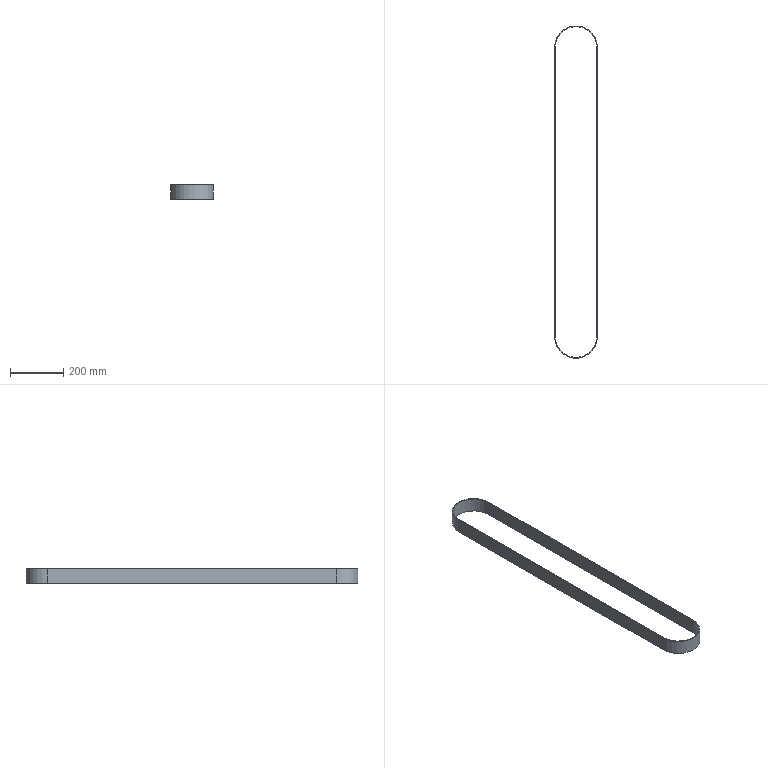Part | STEP file | timing belt 14M-2660L_default | 1 solid | 10 faces | box 161.176 x 1246 x 55 mm | volume 381989 mm3 | plane 6 | cylinder 4 | commonest cylinder face diameters 155.97 x2 161.176 x2
STEP:
#1=CARTESIAN_POINT('',(0.,0.,0.));
#2=DIRECTION('',(0.,0.,1.));
#3=DIRECTION('',(1.,0.,0.));
#4=AXIS2_PLACEMENT_3D('',#1,#2,#3);
#5=CARTESIAN_POINT('',(80.588,0.,-35.));
#6=VERTEX_POINT('',#5);
#7=CARTESIAN_POINT('',(-80.588,0.,-35.));
#8=VERTEX_POINT('',#7);
#9=CARTESIAN_POINT('',(0.,0.,-35.));
#10=DIRECTION('',(0.,0.,-1.));
#11=DIRECTION('',(-1.,0.,0.));
#12=AXIS2_PLACEMENT_3D('',#9,#10,#11);
#13=CIRCLE('',#12,80.588);
#14=CARTESIAN_POINT('',(0.,0.,20.));
#15=DIRECTION('',(0.,0.,-1.));
#16=DIRECTION('',(-1.,0.,0.));
#17=AXIS2_PLACEMENT_3D('',#14,#15,#16);
#18=CYLINDRICAL_SURFACE('',#17,80.588);
#19=CARTESIAN_POINT('',(0.,55.));
#20=DIRECTION('',(1.,0.));
#21=VECTOR('',#20,1.);
#22=LINE('',#19,#21);
#23=(GEOMETRIC_REPRESENTATION_CONTEXT(2)PARAMETRIC_REPRESENTATION_CONTEXT()REPRESENTATION_CONTEXT('',''));
#24=DEFINITIONAL_REPRESENTATION('',(#22),#23);
#25=PCURVE('',#18,#24);
#26=CARTESIAN_POINT('',(0.,0.,-35.));
#27=DIRECTION('',(0.,0.,-1.));
#28=DIRECTION('',(-1.,0.,0.));
#29=AXIS2_PLACEMENT_3D('',#26,#27,#28);
#30=PLANE('',#29);
#31=CARTESIAN_POINT('',(0.,0.));
#32=DIRECTION('',(1.,0.));
#33=AXIS2_PLACEMENT_2D('',#31,#32);
#34=CIRCLE('',#33,80.588);
#35=(GEOMETRIC_REPRESENTATION_CONTEXT(2)PARAMETRIC_REPRESENTATION_CONTEXT()REPRESENTATION_CONTEXT('',''));
#36=DEFINITIONAL_REPRESENTATION('',(#34),#35);
#37=PCURVE('',#30,#36);
#38=SURFACE_CURVE('',#13,(#25,#37),.PCURVE_S1.);
#39=EDGE_CURVE('',#6,#8,#38,.T.);
#40=ORIENTED_EDGE('',*,*,#39,.F.);
#41=CARTESIAN_POINT('',(80.588,0.,20.));
#42=VERTEX_POINT('',#41);
#43=CARTESIAN_POINT('',(80.588,0.,20.));
#44=DIRECTION('',(0.,0.,-1.));
#45=VECTOR('',#44,1.);
#46=LINE('',#43,#45);
#47=CARTESIAN_POINT('',(3.142,0.));
#48=DIRECTION('',(0.,1.));
#49=VECTOR('',#48,1.);
#50=LINE('',#47,#49);
#51=(GEOMETRIC_REPRESENTATION_CONTEXT(2)PARAMETRIC_REPRESENTATION_CONTEXT()REPRESENTATION_CONTEXT('',''));
#52=DEFINITIONAL_REPRESENTATION('',(#50),#51);
#53=PCURVE('',#18,#52);
#54=CARTESIAN_POINT('',(80.588,1085.,20.));
#55=DIRECTION('',(1.,0.,0.));
#56=DIRECTION('',(0.,1.,0.));
#57=AXIS2_PLACEMENT_3D('',#54,#55,#56);
#58=PLANE('',#57);
#59=CARTESIAN_POINT('',(-1085.,0.));
#60=DIRECTION('',(0.,-1.));
#61=VECTOR('',#60,1.);
#62=LINE('',#59,#61);
#63=(GEOMETRIC_REPRESENTATION_CONTEXT(2)PARAMETRIC_REPRESENTATION_CONTEXT()REPRESENTATION_CONTEXT('',''));
#64=DEFINITIONAL_REPRESENTATION('',(#62),#63);
#65=PCURVE('',#58,#64);
#66=SURFACE_CURVE('',#46,(#53,#65),.PCURVE_S1.);
#67=EDGE_CURVE('',#42,#6,#66,.T.);
#68=ORIENTED_EDGE('',*,*,#67,.F.);
#69=CARTESIAN_POINT('',(-80.588,0.,20.));
#70=VERTEX_POINT('',#69);
#71=CARTESIAN_POINT('',(0.,0.,20.));
#72=DIRECTION('',(0.,0.,-1.));
#73=DIRECTION('',(-1.,0.,0.));
#74=AXIS2_PLACEMENT_3D('',#71,#72,#73);
#75=CIRCLE('',#74,80.588);
#76=CARTESIAN_POINT('',(0.,0.));
#77=DIRECTION('',(1.,0.));
#78=VECTOR('',#77,1.);
#79=LINE('',#76,#78);
#80=(GEOMETRIC_REPRESENTATION_CONTEXT(2)PARAMETRIC_REPRESENTATION_CONTEXT()REPRESENTATION_CONTEXT('',''));
#81=DEFINITIONAL_REPRESENTATION('',(#79),#80);
#82=PCURVE('',#18,#81);
#83=CARTESIAN_POINT('',(0.,0.,20.));
#84=DIRECTION('',(0.,0.,-1.));
#85=DIRECTION('',(-1.,0.,0.));
#86=AXIS2_PLACEMENT_3D('',#83,#84,#85);
#87=PLANE('',#86);
#88=CARTESIAN_POINT('',(0.,0.));
#89=DIRECTION('',(1.,0.));
#90=AXIS2_PLACEMENT_2D('',#88,#89);
#91=CIRCLE('',#90,80.588);
#92=(GEOMETRIC_REPRESENTATION_CONTEXT(2)PARAMETRIC_REPRESENTATION_CONTEXT()REPRESENTATION_CONTEXT('',''));
#93=DEFINITIONAL_REPRESENTATION('',(#91),#92);
#94=PCURVE('',#87,#93);
#95=SURFACE_CURVE('',#75,(#82,#94),.PCURVE_S1.);
#96=EDGE_CURVE('',#42,#70,#95,.T.);
#97=ORIENTED_EDGE('',*,*,#96,.T.);
#98=CARTESIAN_POINT('',(-80.588,0.,20.));
#99=DIRECTION('',(0.,0.,-1.));
#100=VECTOR('',#99,1.);
#101=LINE('',#98,#100);
#102=CARTESIAN_POINT('',(6.283,0.));
#103=DIRECTION('',(0.,1.));
#104=VECTOR('',#103,1.);
#105=LINE('',#102,#104);
#106=(GEOMETRIC_REPRESENTATION_CONTEXT(2)PARAMETRIC_REPRESENTATION_CONTEXT()REPRESENTATION_CONTEXT('',''));
#107=DEFINITIONAL_REPRESENTATION('',(#105),#106);
#108=PCURVE('',#18,#107);
#109=CARTESIAN_POINT('',(-80.588,0.,20.));
#110=DIRECTION('',(-1.,0.,0.));
#111=DIRECTION('',(0.,0.,1.));
#112=AXIS2_PLACEMENT_3D('',#109,#110,#111);
#113=PLANE('',#112);
#114=CARTESIAN_POINT('',(0.,0.));
#115=DIRECTION('',(-1.,0.));
#116=VECTOR('',#115,1.);
#117=LINE('',#114,#116);
#118=(GEOMETRIC_REPRESENTATION_CONTEXT(2)PARAMETRIC_REPRESENTATION_CONTEXT()REPRESENTATION_CONTEXT('',''));
#119=DEFINITIONAL_REPRESENTATION('',(#117),#118);
#120=PCURVE('',#113,#119);
#121=SURFACE_CURVE('',#101,(#108,#120),.PCURVE_S1.);
#122=EDGE_CURVE('',#70,#8,#121,.T.);
#123=ORIENTED_EDGE('',*,*,#122,.T.);
#124=EDGE_LOOP('',(#40,#68,#97,#123));
#125=FACE_BOUND('',#124,.T.);
#126=ADVANCED_FACE('',(#125),#18,.T.);
#127=CARTESIAN_POINT('',(80.588,1085.,-35.));
#128=VERTEX_POINT('',#127);
#129=CARTESIAN_POINT('',(80.588,1085.,-35.));
#130=DIRECTION('',(0.,-1.,0.));
#131=VECTOR('',#130,1.);
#132=LINE('',#129,#131);
#133=CARTESIAN_POINT('',(0.,-55.));
#134=DIRECTION('',(-1.,0.));
#135=VECTOR('',#134,1.);
#136=LINE('',#133,#135);
#137=(GEOMETRIC_REPRESENTATION_CONTEXT(2)PARAMETRIC_REPRESENTATION_CONTEXT()REPRESENTATION_CONTEXT('',''));
#138=DEFINITIONAL_REPRESENTATION('',(#136),#137);
#139=PCURVE('',#58,#138);
#140=CARTESIAN_POINT('',(-80.588,1085.));
#141=DIRECTION('',(0.,-1.));
#142=VECTOR('',#141,1.);
#143=LINE('',#140,#142);
#144=(GEOMETRIC_REPRESENTATION_CONTEXT(2)PARAMETRIC_REPRESENTATION_CONTEXT()REPRESENTATION_CONTEXT('',''));
#145=DEFINITIONAL_REPRESENTATION('',(#143),#144);
#146=PCURVE('',#30,#145);
#147=SURFACE_CURVE('',#132,(#139,#146),.PCURVE_S1.);
#148=EDGE_CURVE('',#128,#6,#147,.T.);
#149=ORIENTED_EDGE('',*,*,#148,.F.);
#150=CARTESIAN_POINT('',(80.588,1085.,20.));
#151=VERTEX_POINT('',#150);
#152=CARTESIAN_POINT('',(80.588,1085.,20.));
#153=DIRECTION('',(0.,0.,-1.));
#154=VECTOR('',#153,1.);
#155=LINE('',#152,#154);
#156=CARTESIAN_POINT('',(0.,0.));
#157=DIRECTION('',(0.,-1.));
#158=VECTOR('',#157,1.);
#159=LINE('',#156,#158);
#160=(GEOMETRIC_REPRESENTATION_CONTEXT(2)PARAMETRIC_REPRESENTATION_CONTEXT()REPRESENTATION_CONTEXT('',''));
#161=DEFINITIONAL_REPRESENTATION('',(#159),#160);
#162=PCURVE('',#58,#161);
#163=CARTESIAN_POINT('',(0.,1085.,20.));
#164=DIRECTION('',(0.,0.,-1.));
#165=DIRECTION('',(-1.,0.,0.));
#166=AXIS2_PLACEMENT_3D('',#163,#164,#165);
#167=CYLINDRICAL_SURFACE('',#166,80.588);
#168=CARTESIAN_POINT('',(3.142,0.));
#169=DIRECTION('',(0.,1.));
#170=VECTOR('',#169,1.);
#171=LINE('',#168,#170);
#172=(GEOMETRIC_REPRESENTATION_CONTEXT(2)PARAMETRIC_REPRESENTATION_CONTEXT()REPRESENTATION_CONTEXT('',''));
#173=DEFINITIONAL_REPRESENTATION('',(#171),#172);
#174=PCURVE('',#167,#173);
#175=SURFACE_CURVE('',#155,(#162,#174),.PCURVE_S1.);
#176=EDGE_CURVE('',#151,#128,#175,.T.);
#177=ORIENTED_EDGE('',*,*,#176,.F.);
#178=CARTESIAN_POINT('',(80.588,1085.,20.));
#179=DIRECTION('',(0.,-1.,0.));
#180=VECTOR('',#179,1.);
#181=LINE('',#178,#180);
#182=CARTESIAN_POINT('',(0.,0.));
#183=DIRECTION('',(-1.,0.));
#184=VECTOR('',#183,1.);
#185=LINE('',#182,#184);
#186=(GEOMETRIC_REPRESENTATION_CONTEXT(2)PARAMETRIC_REPRESENTATION_CONTEXT()REPRESENTATION_CONTEXT('',''));
#187=DEFINITIONAL_REPRESENTATION('',(#185),#186);
#188=PCURVE('',#58,#187);
#189=CARTESIAN_POINT('',(-80.588,1085.));
#190=DIRECTION('',(0.,-1.));
#191=VECTOR('',#190,1.);
#192=LINE('',#189,#191);
#193=(GEOMETRIC_REPRESENTATION_CONTEXT(2)PARAMETRIC_REPRESENTATION_CONTEXT()REPRESENTATION_CONTEXT('',''));
#194=DEFINITIONAL_REPRESENTATION('',(#192),#193);
#195=PCURVE('',#87,#194);
#196=SURFACE_CURVE('',#181,(#188,#195),.PCURVE_S1.);
#197=EDGE_CURVE('',#151,#42,#196,.T.);
#198=ORIENTED_EDGE('',*,*,#197,.T.);
#199=ORIENTED_EDGE('',*,*,#67,.T.);
#200=EDGE_LOOP('',(#149,#177,#198,#199));
#201=FACE_BOUND('',#200,.T.);
#202=ADVANCED_FACE('',(#201),#58,.T.);
#203=CARTESIAN_POINT('',(-80.588,1085.,-35.));
#204=VERTEX_POINT('',#203);
#205=CARTESIAN_POINT('',(0.,1085.,-35.));
#206=DIRECTION('',(0.,0.,-1.));
#207=DIRECTION('',(-1.,0.,0.));
#208=AXIS2_PLACEMENT_3D('',#205,#206,#207);
#209=CIRCLE('',#208,80.588);
#210=CARTESIAN_POINT('',(0.,55.));
#211=DIRECTION('',(1.,0.));
#212=VECTOR('',#211,1.);
#213=LINE('',#210,#212);
#214=(GEOMETRIC_REPRESENTATION_CONTEXT(2)PARAMETRIC_REPRESENTATION_CONTEXT()REPRESENTATION_CONTEXT('',''));
#215=DEFINITIONAL_REPRESENTATION('',(#213),#214);
#216=PCURVE('',#167,#215);
#217=CARTESIAN_POINT('',(0.,1085.));
#218=DIRECTION('',(1.,0.));
#219=AXIS2_PLACEMENT_2D('',#217,#218);
#220=CIRCLE('',#219,80.588);
#221=(GEOMETRIC_REPRESENTATION_CONTEXT(2)PARAMETRIC_REPRESENTATION_CONTEXT()REPRESENTATION_CONTEXT('',''));
#222=DEFINITIONAL_REPRESENTATION('',(#220),#221);
#223=PCURVE('',#30,#222);
#224=SURFACE_CURVE('',#209,(#216,#223),.PCURVE_S1.);
#225=EDGE_CURVE('',#204,#128,#224,.T.);
#226=ORIENTED_EDGE('',*,*,#225,.F.);
#227=CARTESIAN_POINT('',(-80.588,1085.,20.));
#228=VERTEX_POINT('',#227);
#229=CARTESIAN_POINT('',(-80.588,1085.,20.));
#230=DIRECTION('',(0.,0.,-1.));
#231=VECTOR('',#230,1.);
#232=LINE('',#229,#231);
#233=CARTESIAN_POINT('',(0.,0.));
#234=DIRECTION('',(0.,1.));
#235=VECTOR('',#234,1.);
#236=LINE('',#233,#235);
#237=(GEOMETRIC_REPRESENTATION_CONTEXT(2)PARAMETRIC_REPRESENTATION_CONTEXT()REPRESENTATION_CONTEXT('',''));
#238=DEFINITIONAL_REPRESENTATION('',(#236),#237);
#239=PCURVE('',#167,#238);
#240=CARTESIAN_POINT('',(0.,1085.));
#241=DIRECTION('',(-1.,0.));
#242=VECTOR('',#241,1.);
#243=LINE('',#240,#242);
#244=(GEOMETRIC_REPRESENTATION_CONTEXT(2)PARAMETRIC_REPRESENTATION_CONTEXT()REPRESENTATION_CONTEXT('',''));
#245=DEFINITIONAL_REPRESENTATION('',(#243),#244);
#246=PCURVE('',#113,#245);
#247=SURFACE_CURVE('',#232,(#239,#246),.PCURVE_S1.);
#248=EDGE_CURVE('',#228,#204,#247,.T.);
#249=ORIENTED_EDGE('',*,*,#248,.F.);
#250=CARTESIAN_POINT('',(0.,1085.,20.));
#251=DIRECTION('',(0.,0.,-1.));
#252=DIRECTION('',(-1.,0.,0.));
#253=AXIS2_PLACEMENT_3D('',#250,#251,#252);
#254=CIRCLE('',#253,80.588);
#255=CARTESIAN_POINT('',(0.,0.));
#256=DIRECTION('',(1.,0.));
#257=VECTOR('',#256,1.);
#258=LINE('',#255,#257);
#259=(GEOMETRIC_REPRESENTATION_CONTEXT(2)PARAMETRIC_REPRESENTATION_CONTEXT()REPRESENTATION_CONTEXT('',''));
#260=DEFINITIONAL_REPRESENTATION('',(#258),#259);
#261=PCURVE('',#167,#260);
#262=CARTESIAN_POINT('',(0.,1085.));
#263=DIRECTION('',(1.,0.));
#264=AXIS2_PLACEMENT_2D('',#262,#263);
#265=CIRCLE('',#264,80.588);
#266=(GEOMETRIC_REPRESENTATION_CONTEXT(2)PARAMETRIC_REPRESENTATION_CONTEXT()REPRESENTATION_CONTEXT('',''));
#267=DEFINITIONAL_REPRESENTATION('',(#265),#266);
#268=PCURVE('',#87,#267);
#269=SURFACE_CURVE('',#254,(#261,#268),.PCURVE_S1.);
#270=EDGE_CURVE('',#228,#151,#269,.T.);
#271=ORIENTED_EDGE('',*,*,#270,.T.);
#272=ORIENTED_EDGE('',*,*,#176,.T.);
#273=EDGE_LOOP('',(#226,#249,#271,#272));
#274=FACE_BOUND('',#273,.T.);
#275=ADVANCED_FACE('',(#274),#167,.T.);
#276=CARTESIAN_POINT('',(-80.588,0.,-35.));
#277=DIRECTION('',(0.,1.,0.));
#278=VECTOR('',#277,1.);
#279=LINE('',#276,#278);
#280=CARTESIAN_POINT('',(-55.,0.));
#281=DIRECTION('',(0.,1.));
#282=VECTOR('',#281,1.);
#283=LINE('',#280,#282);
#284=(GEOMETRIC_REPRESENTATION_CONTEXT(2)PARAMETRIC_REPRESENTATION_CONTEXT()REPRESENTATION_CONTEXT('',''));
#285=DEFINITIONAL_REPRESENTATION('',(#283),#284);
#286=PCURVE('',#113,#285);
#287=CARTESIAN_POINT('',(80.588,0.));
#288=DIRECTION('',(0.,1.));
#289=VECTOR('',#288,1.);
#290=LINE('',#287,#289);
#291=(GEOMETRIC_REPRESENTATION_CONTEXT(2)PARAMETRIC_REPRESENTATION_CONTEXT()REPRESENTATION_CONTEXT('',''));
#292=DEFINITIONAL_REPRESENTATION('',(#290),#291);
#293=PCURVE('',#30,#292);
#294=SURFACE_CURVE('',#279,(#286,#293),.PCURVE_S1.);
#295=EDGE_CURVE('',#8,#204,#294,.T.);
#296=ORIENTED_EDGE('',*,*,#295,.F.);
#297=ORIENTED_EDGE('',*,*,#122,.F.);
#298=CARTESIAN_POINT('',(-80.588,0.,20.));
#299=DIRECTION('',(0.,1.,0.));
#300=VECTOR('',#299,1.);
#301=LINE('',#298,#300);
#302=CARTESIAN_POINT('',(0.,0.));
#303=DIRECTION('',(0.,1.));
#304=VECTOR('',#303,1.);
#305=LINE('',#302,#304);
#306=(GEOMETRIC_REPRESENTATION_CONTEXT(2)PARAMETRIC_REPRESENTATION_CONTEXT()REPRESENTATION_CONTEXT('',''));
#307=DEFINITIONAL_REPRESENTATION('',(#305),#306);
#308=PCURVE('',#113,#307);
#309=CARTESIAN_POINT('',(80.588,0.));
#310=DIRECTION('',(0.,1.));
#311=VECTOR('',#310,1.);
#312=LINE('',#309,#311);
#313=(GEOMETRIC_REPRESENTATION_CONTEXT(2)PARAMETRIC_REPRESENTATION_CONTEXT()REPRESENTATION_CONTEXT('',''));
#314=DEFINITIONAL_REPRESENTATION('',(#312),#313);
#315=PCURVE('',#87,#314);
#316=SURFACE_CURVE('',#301,(#308,#315),.PCURVE_S1.);
#317=EDGE_CURVE('',#70,#228,#316,.T.);
#318=ORIENTED_EDGE('',*,*,#317,.T.);
#319=ORIENTED_EDGE('',*,*,#248,.T.);
#320=EDGE_LOOP('',(#296,#297,#318,#319));
#321=FACE_BOUND('',#320,.T.);
#322=ADVANCED_FACE('',(#321),#113,.T.);
#323=CARTESIAN_POINT('',(77.985,1085.,20.));
#324=VERTEX_POINT('',#323);
#325=CARTESIAN_POINT('',(77.985,0.,20.));
#326=VERTEX_POINT('',#325);
#327=CARTESIAN_POINT('',(77.985,0.,20.));
#328=DIRECTION('',(0.,-1.,0.));
#329=VECTOR('',#328,1.);
#330=LINE('',#327,#329);
#331=CARTESIAN_POINT('',(-77.985,0.));
#332=DIRECTION('',(0.,-1.));
#333=VECTOR('',#332,1.);
#334=LINE('',#331,#333);
#335=(GEOMETRIC_REPRESENTATION_CONTEXT(2)PARAMETRIC_REPRESENTATION_CONTEXT()REPRESENTATION_CONTEXT('',''));
#336=DEFINITIONAL_REPRESENTATION('',(#334),#335);
#337=PCURVE('',#87,#336);
#338=CARTESIAN_POINT('',(77.985,0.,20.));
#339=DIRECTION('',(1.,0.,0.));
#340=DIRECTION('',(0.,0.,-1.));
#341=AXIS2_PLACEMENT_3D('',#338,#339,#340);
#342=PLANE('',#341);
#343=CARTESIAN_POINT('',(0.,0.));
#344=DIRECTION('',(0.,-1.));
#345=VECTOR('',#344,1.);
#346=LINE('',#343,#345);
#347=(GEOMETRIC_REPRESENTATION_CONTEXT(2)PARAMETRIC_REPRESENTATION_CONTEXT()REPRESENTATION_CONTEXT('',''));
#348=DEFINITIONAL_REPRESENTATION('',(#346),#347);
#349=PCURVE('',#342,#348);
#350=SURFACE_CURVE('',#330,(#337,#349),.PCURVE_S1.);
#351=EDGE_CURVE('',#324,#326,#350,.T.);
#352=ORIENTED_EDGE('',*,*,#351,.T.);
#353=CARTESIAN_POINT('',(-77.985,0.,20.));
#354=VERTEX_POINT('',#353);
#355=CARTESIAN_POINT('',(0.,0.,20.));
#356=DIRECTION('',(0.,0.,-1.));
#357=DIRECTION('',(1.,0.,0.));
#358=AXIS2_PLACEMENT_3D('',#355,#356,#357);
#359=CIRCLE('',#358,77.985);
#360=CARTESIAN_POINT('',(0.,0.));
#361=DIRECTION('',(-1.,0.));
#362=AXIS2_PLACEMENT_2D('',#360,#361);
#363=CIRCLE('',#362,77.985);
#364=(GEOMETRIC_REPRESENTATION_CONTEXT(2)PARAMETRIC_REPRESENTATION_CONTEXT()REPRESENTATION_CONTEXT('',''));
#365=DEFINITIONAL_REPRESENTATION('',(#363),#364);
#366=PCURVE('',#87,#365);
#367=CARTESIAN_POINT('',(0.,0.,20.));
#368=DIRECTION('',(0.,0.,-1.));
#369=DIRECTION('',(-1.,0.,0.));
#370=AXIS2_PLACEMENT_3D('',#367,#368,#369);
#371=CYLINDRICAL_SURFACE('',#370,77.985);
#372=CARTESIAN_POINT('',(3.142,0.));
#373=DIRECTION('',(1.,0.));
#374=VECTOR('',#373,1.);
#375=LINE('',#372,#374);
#376=(GEOMETRIC_REPRESENTATION_CONTEXT(2)PARAMETRIC_REPRESENTATION_CONTEXT()REPRESENTATION_CONTEXT('',''));
#377=DEFINITIONAL_REPRESENTATION('',(#375),#376);
#378=PCURVE('',#371,#377);
#379=SURFACE_CURVE('',#359,(#366,#378),.PCURVE_S1.);
#380=EDGE_CURVE('',#326,#354,#379,.T.);
#381=ORIENTED_EDGE('',*,*,#380,.T.);
#382=CARTESIAN_POINT('',(-77.985,1085.,20.));
#383=VERTEX_POINT('',#382);
#384=CARTESIAN_POINT('',(-77.985,1085.,20.));
#385=DIRECTION('',(0.,1.,0.));
#386=VECTOR('',#385,1.);
#387=LINE('',#384,#386);
#388=CARTESIAN_POINT('',(77.985,1085.));
#389=DIRECTION('',(0.,1.));
#390=VECTOR('',#389,1.);
#391=LINE('',#388,#390);
#392=(GEOMETRIC_REPRESENTATION_CONTEXT(2)PARAMETRIC_REPRESENTATION_CONTEXT()REPRESENTATION_CONTEXT('',''));
#393=DEFINITIONAL_REPRESENTATION('',(#391),#392);
#394=PCURVE('',#87,#393);
#395=CARTESIAN_POINT('',(-77.985,1085.,20.));
#396=DIRECTION('',(-1.,0.,0.));
#397=DIRECTION('',(0.,-1.,0.));
#398=AXIS2_PLACEMENT_3D('',#395,#396,#397);
#399=PLANE('',#398);
#400=CARTESIAN_POINT('',(0.,0.));
#401=DIRECTION('',(-1.,0.));
#402=VECTOR('',#401,1.);
#403=LINE('',#400,#402);
#404=(GEOMETRIC_REPRESENTATION_CONTEXT(2)PARAMETRIC_REPRESENTATION_CONTEXT()REPRESENTATION_CONTEXT('',''));
#405=DEFINITIONAL_REPRESENTATION('',(#403),#404);
#406=PCURVE('',#399,#405);
#407=SURFACE_CURVE('',#387,(#394,#406),.PCURVE_S1.);
#408=EDGE_CURVE('',#354,#383,#407,.T.);
#409=ORIENTED_EDGE('',*,*,#408,.T.);
#410=CARTESIAN_POINT('',(0.,1085.,20.));
#411=DIRECTION('',(0.,0.,-1.));
#412=DIRECTION('',(1.,0.,0.));
#413=AXIS2_PLACEMENT_3D('',#410,#411,#412);
#414=CIRCLE('',#413,77.985);
#415=CARTESIAN_POINT('',(0.,1085.));
#416=DIRECTION('',(-1.,0.));
#417=AXIS2_PLACEMENT_2D('',#415,#416);
#418=CIRCLE('',#417,77.985);
#419=(GEOMETRIC_REPRESENTATION_CONTEXT(2)PARAMETRIC_REPRESENTATION_CONTEXT()REPRESENTATION_CONTEXT('',''));
#420=DEFINITIONAL_REPRESENTATION('',(#418),#419);
#421=PCURVE('',#87,#420);
#422=CARTESIAN_POINT('',(0.,1085.,20.));
#423=DIRECTION('',(0.,0.,-1.));
#424=DIRECTION('',(-1.,0.,0.));
#425=AXIS2_PLACEMENT_3D('',#422,#423,#424);
#426=CYLINDRICAL_SURFACE('',#425,77.985);
#427=CARTESIAN_POINT('',(-3.142,0.));
#428=DIRECTION('',(1.,0.));
#429=VECTOR('',#428,1.);
#430=LINE('',#427,#429);
#431=(GEOMETRIC_REPRESENTATION_CONTEXT(2)PARAMETRIC_REPRESENTATION_CONTEXT()REPRESENTATION_CONTEXT('',''));
#432=DEFINITIONAL_REPRESENTATION('',(#430),#431);
#433=PCURVE('',#426,#432);
#434=SURFACE_CURVE('',#414,(#421,#433),.PCURVE_S1.);
#435=EDGE_CURVE('',#383,#324,#434,.T.);
#436=ORIENTED_EDGE('',*,*,#435,.T.);
#437=EDGE_LOOP('',(#352,#381,#409,#436));
#438=FACE_BOUND('',#437,.T.);
#439=ORIENTED_EDGE('',*,*,#96,.F.);
#440=ORIENTED_EDGE('',*,*,#197,.F.);
#441=ORIENTED_EDGE('',*,*,#270,.F.);
#442=ORIENTED_EDGE('',*,*,#317,.F.);
#443=EDGE_LOOP('',(#439,#440,#441,#442));
#444=FACE_BOUND('',#443,.T.);
#445=ADVANCED_FACE('',(#438,#444),#87,.F.);
#446=CARTESIAN_POINT('',(77.985,0.,-35.));
#447=VERTEX_POINT('',#446);
#448=CARTESIAN_POINT('',(-77.985,0.,-35.));
#449=VERTEX_POINT('',#448);
#450=CARTESIAN_POINT('',(0.,0.,-35.));
#451=DIRECTION('',(0.,0.,-1.));
#452=DIRECTION('',(1.,0.,0.));
#453=AXIS2_PLACEMENT_3D('',#450,#451,#452);
#454=CIRCLE('',#453,77.985);
#455=CARTESIAN_POINT('',(0.,0.));
#456=DIRECTION('',(-1.,0.));
#457=AXIS2_PLACEMENT_2D('',#455,#456);
#458=CIRCLE('',#457,77.985);
#459=(GEOMETRIC_REPRESENTATION_CONTEXT(2)PARAMETRIC_REPRESENTATION_CONTEXT()REPRESENTATION_CONTEXT('',''));
#460=DEFINITIONAL_REPRESENTATION('',(#458),#459);
#461=PCURVE('',#30,#460);
#462=CARTESIAN_POINT('',(3.142,55.));
#463=DIRECTION('',(1.,0.));
#464=VECTOR('',#463,1.);
#465=LINE('',#462,#464);
#466=(GEOMETRIC_REPRESENTATION_CONTEXT(2)PARAMETRIC_REPRESENTATION_CONTEXT()REPRESENTATION_CONTEXT('',''));
#467=DEFINITIONAL_REPRESENTATION('',(#465),#466);
#468=PCURVE('',#371,#467);
#469=SURFACE_CURVE('',#454,(#461,#468),.PCURVE_S1.);
#470=EDGE_CURVE('',#447,#449,#469,.T.);
#471=ORIENTED_EDGE('',*,*,#470,.F.);
#472=CARTESIAN_POINT('',(77.985,1085.,-35.));
#473=VERTEX_POINT('',#472);
#474=CARTESIAN_POINT('',(77.985,0.,-35.));
#475=DIRECTION('',(0.,-1.,0.));
#476=VECTOR('',#475,1.);
#477=LINE('',#474,#476);
#478=CARTESIAN_POINT('',(-77.985,0.));
#479=DIRECTION('',(0.,-1.));
#480=VECTOR('',#479,1.);
#481=LINE('',#478,#480);
#482=(GEOMETRIC_REPRESENTATION_CONTEXT(2)PARAMETRIC_REPRESENTATION_CONTEXT()REPRESENTATION_CONTEXT('',''));
#483=DEFINITIONAL_REPRESENTATION('',(#481),#482);
#484=PCURVE('',#30,#483);
#485=CARTESIAN_POINT('',(55.,0.));
#486=DIRECTION('',(0.,-1.));
#487=VECTOR('',#486,1.);
#488=LINE('',#485,#487);
#489=(GEOMETRIC_REPRESENTATION_CONTEXT(2)PARAMETRIC_REPRESENTATION_CONTEXT()REPRESENTATION_CONTEXT('',''));
#490=DEFINITIONAL_REPRESENTATION('',(#488),#489);
#491=PCURVE('',#342,#490);
#492=SURFACE_CURVE('',#477,(#484,#491),.PCURVE_S1.);
#493=EDGE_CURVE('',#473,#447,#492,.T.);
#494=ORIENTED_EDGE('',*,*,#493,.F.);
#495=CARTESIAN_POINT('',(-77.985,1085.,-35.));
#496=VERTEX_POINT('',#495);
#497=CARTESIAN_POINT('',(0.,1085.,-35.));
#498=DIRECTION('',(0.,0.,-1.));
#499=DIRECTION('',(1.,0.,0.));
#500=AXIS2_PLACEMENT_3D('',#497,#498,#499);
#501=CIRCLE('',#500,77.985);
#502=CARTESIAN_POINT('',(0.,1085.));
#503=DIRECTION('',(-1.,0.));
#504=AXIS2_PLACEMENT_2D('',#502,#503);
#505=CIRCLE('',#504,77.985);
#506=(GEOMETRIC_REPRESENTATION_CONTEXT(2)PARAMETRIC_REPRESENTATION_CONTEXT()REPRESENTATION_CONTEXT('',''));
#507=DEFINITIONAL_REPRESENTATION('',(#505),#506);
#508=PCURVE('',#30,#507);
#509=CARTESIAN_POINT('',(-3.142,55.));
#510=DIRECTION('',(1.,0.));
#511=VECTOR('',#510,1.);
#512=LINE('',#509,#511);
#513=(GEOMETRIC_REPRESENTATION_CONTEXT(2)PARAMETRIC_REPRESENTATION_CONTEXT()REPRESENTATION_CONTEXT('',''));
#514=DEFINITIONAL_REPRESENTATION('',(#512),#513);
#515=PCURVE('',#426,#514);
#516=SURFACE_CURVE('',#501,(#508,#515),.PCURVE_S1.);
#517=EDGE_CURVE('',#496,#473,#516,.T.);
#518=ORIENTED_EDGE('',*,*,#517,.F.);
#519=CARTESIAN_POINT('',(-77.985,1085.,-35.));
#520=DIRECTION('',(0.,1.,0.));
#521=VECTOR('',#520,1.);
#522=LINE('',#519,#521);
#523=CARTESIAN_POINT('',(77.985,1085.));
#524=DIRECTION('',(0.,1.));
#525=VECTOR('',#524,1.);
#526=LINE('',#523,#525);
#527=(GEOMETRIC_REPRESENTATION_CONTEXT(2)PARAMETRIC_REPRESENTATION_CONTEXT()REPRESENTATION_CONTEXT('',''));
#528=DEFINITIONAL_REPRESENTATION('',(#526),#527);
#529=PCURVE('',#30,#528);
#530=CARTESIAN_POINT('',(0.,-55.));
#531=DIRECTION('',(-1.,0.));
#532=VECTOR('',#531,1.);
#533=LINE('',#530,#532);
#534=(GEOMETRIC_REPRESENTATION_CONTEXT(2)PARAMETRIC_REPRESENTATION_CONTEXT()REPRESENTATION_CONTEXT('',''));
#535=DEFINITIONAL_REPRESENTATION('',(#533),#534);
#536=PCURVE('',#399,#535);
#537=SURFACE_CURVE('',#522,(#529,#536),.PCURVE_S1.);
#538=EDGE_CURVE('',#449,#496,#537,.T.);
#539=ORIENTED_EDGE('',*,*,#538,.F.);
#540=EDGE_LOOP('',(#471,#494,#518,#539));
#541=FACE_BOUND('',#540,.T.);
#542=ORIENTED_EDGE('',*,*,#39,.T.);
#543=ORIENTED_EDGE('',*,*,#295,.T.);
#544=ORIENTED_EDGE('',*,*,#225,.T.);
#545=ORIENTED_EDGE('',*,*,#148,.T.);
#546=EDGE_LOOP('',(#542,#543,#544,#545));
#547=FACE_BOUND('',#546,.T.);
#548=ADVANCED_FACE('',(#541,#547),#30,.T.);
#549=CARTESIAN_POINT('',(77.985,0.,20.));
#550=DIRECTION('',(0.,0.,-1.));
#551=VECTOR('',#550,1.);
#552=LINE('',#549,#551);
#553=CARTESIAN_POINT('',(3.142,0.));
#554=DIRECTION('',(0.,1.));
#555=VECTOR('',#554,1.);
#556=LINE('',#553,#555);
#557=(GEOMETRIC_REPRESENTATION_CONTEXT(2)PARAMETRIC_REPRESENTATION_CONTEXT()REPRESENTATION_CONTEXT('',''));
#558=DEFINITIONAL_REPRESENTATION('',(#556),#557);
#559=PCURVE('',#371,#558);
#560=CARTESIAN_POINT('',(0.,0.));
#561=DIRECTION('',(1.,0.));
#562=VECTOR('',#561,1.);
#563=LINE('',#560,#562);
#564=(GEOMETRIC_REPRESENTATION_CONTEXT(2)PARAMETRIC_REPRESENTATION_CONTEXT()REPRESENTATION_CONTEXT('',''));
#565=DEFINITIONAL_REPRESENTATION('',(#563),#564);
#566=PCURVE('',#342,#565);
#567=SURFACE_CURVE('',#552,(#559,#566),.PCURVE_S1.);
#568=EDGE_CURVE('',#326,#447,#567,.T.);
#569=ORIENTED_EDGE('',*,*,#568,.F.);
#570=ORIENTED_EDGE('',*,*,#380,.T.);
#571=CARTESIAN_POINT('',(-77.985,0.,20.));
#572=DIRECTION('',(0.,0.,-1.));
#573=VECTOR('',#572,1.);
#574=LINE('',#571,#573);
#575=CARTESIAN_POINT('',(6.283,0.));
#576=DIRECTION('',(0.,1.));
#577=VECTOR('',#576,1.);
#578=LINE('',#575,#577);
#579=(GEOMETRIC_REPRESENTATION_CONTEXT(2)PARAMETRIC_REPRESENTATION_CONTEXT()REPRESENTATION_CONTEXT('',''));
#580=DEFINITIONAL_REPRESENTATION('',(#578),#579);
#581=PCURVE('',#371,#580);
#582=CARTESIAN_POINT('',(1085.,0.));
#583=DIRECTION('',(0.,-1.));
#584=VECTOR('',#583,1.);
#585=LINE('',#582,#584);
#586=(GEOMETRIC_REPRESENTATION_CONTEXT(2)PARAMETRIC_REPRESENTATION_CONTEXT()REPRESENTATION_CONTEXT('',''));
#587=DEFINITIONAL_REPRESENTATION('',(#585),#586);
#588=PCURVE('',#399,#587);
#589=SURFACE_CURVE('',#574,(#581,#588),.PCURVE_S1.);
#590=EDGE_CURVE('',#354,#449,#589,.T.);
#591=ORIENTED_EDGE('',*,*,#590,.T.);
#592=ORIENTED_EDGE('',*,*,#470,.F.);
#593=EDGE_LOOP('',(#569,#570,#591,#592));
#594=FACE_BOUND('',#593,.F.);
#595=ADVANCED_FACE('',(#594),#371,.F.);
#596=ORIENTED_EDGE('',*,*,#493,.T.);
#597=ORIENTED_EDGE('',*,*,#568,.F.);
#598=ORIENTED_EDGE('',*,*,#351,.F.);
#599=CARTESIAN_POINT('',(77.985,1085.,20.));
#600=DIRECTION('',(0.,0.,-1.));
#601=VECTOR('',#600,1.);
#602=LINE('',#599,#601);
#603=CARTESIAN_POINT('',(0.,1085.));
#604=DIRECTION('',(1.,0.));
#605=VECTOR('',#604,1.);
#606=LINE('',#603,#605);
#607=(GEOMETRIC_REPRESENTATION_CONTEXT(2)PARAMETRIC_REPRESENTATION_CONTEXT()REPRESENTATION_CONTEXT('',''));
#608=DEFINITIONAL_REPRESENTATION('',(#606),#607);
#609=PCURVE('',#342,#608);
#610=CARTESIAN_POINT('',(3.142,0.));
#611=DIRECTION('',(0.,1.));
#612=VECTOR('',#611,1.);
#613=LINE('',#610,#612);
#614=(GEOMETRIC_REPRESENTATION_CONTEXT(2)PARAMETRIC_REPRESENTATION_CONTEXT()REPRESENTATION_CONTEXT('',''));
#615=DEFINITIONAL_REPRESENTATION('',(#613),#614);
#616=PCURVE('',#426,#615);
#617=SURFACE_CURVE('',#602,(#609,#616),.PCURVE_S1.);
#618=EDGE_CURVE('',#324,#473,#617,.T.);
#619=ORIENTED_EDGE('',*,*,#618,.T.);
#620=EDGE_LOOP('',(#596,#597,#598,#619));
#621=FACE_BOUND('',#620,.T.);
#622=ADVANCED_FACE('',(#621),#342,.F.);
#623=CARTESIAN_POINT('',(-77.985,1085.,20.));
#624=DIRECTION('',(0.,0.,-1.));
#625=VECTOR('',#624,1.);
#626=LINE('',#623,#625);
#627=CARTESIAN_POINT('',(0.,0.));
#628=DIRECTION('',(0.,1.));
#629=VECTOR('',#628,1.);
#630=LINE('',#627,#629);
#631=(GEOMETRIC_REPRESENTATION_CONTEXT(2)PARAMETRIC_REPRESENTATION_CONTEXT()REPRESENTATION_CONTEXT('',''));
#632=DEFINITIONAL_REPRESENTATION('',(#630),#631);
#633=PCURVE('',#426,#632);
#634=CARTESIAN_POINT('',(0.,0.));
#635=DIRECTION('',(0.,-1.));
#636=VECTOR('',#635,1.);
#637=LINE('',#634,#636);
#638=(GEOMETRIC_REPRESENTATION_CONTEXT(2)PARAMETRIC_REPRESENTATION_CONTEXT()REPRESENTATION_CONTEXT('',''));
#639=DEFINITIONAL_REPRESENTATION('',(#637),#638);
#640=PCURVE('',#399,#639);
#641=SURFACE_CURVE('',#626,(#633,#640),.PCURVE_S1.);
#642=EDGE_CURVE('',#383,#496,#641,.T.);
#643=ORIENTED_EDGE('',*,*,#642,.F.);
#644=ORIENTED_EDGE('',*,*,#435,.T.);
#645=ORIENTED_EDGE('',*,*,#618,.T.);
#646=ORIENTED_EDGE('',*,*,#517,.F.);
#647=EDGE_LOOP('',(#643,#644,#645,#646));
#648=FACE_BOUND('',#647,.F.);
#649=ADVANCED_FACE('',(#648),#426,.F.);
#650=ORIENTED_EDGE('',*,*,#538,.T.);
#651=ORIENTED_EDGE('',*,*,#642,.F.);
#652=ORIENTED_EDGE('',*,*,#408,.F.);
#653=ORIENTED_EDGE('',*,*,#590,.T.);
#654=EDGE_LOOP('',(#650,#651,#652,#653));
#655=FACE_BOUND('',#654,.T.);
#656=ADVANCED_FACE('',(#655),#399,.F.);
#657=CLOSED_SHELL('',(#126,#202,#275,#322,#445,#548,#595,#622,#649,#656));
#658=MANIFOLD_SOLID_BREP('',#657);
#659=(LENGTH_UNIT()NAMED_UNIT(*)SI_UNIT(.MILLI.,.METRE.));
#660=UNCERTAINTY_MEASURE_WITH_UNIT(LENGTH_MEASURE(0.0000001),#659,'','');
#661=(NAMED_UNIT(*)PLANE_ANGLE_UNIT()SI_UNIT($,.RADIAN.));
#662=(NAMED_UNIT(*)SI_UNIT($,.STERADIAN.)SOLID_ANGLE_UNIT());
#663=(GEOMETRIC_REPRESENTATION_CONTEXT(3)GLOBAL_UNCERTAINTY_ASSIGNED_CONTEXT((#660))GLOBAL_UNIT_ASSIGNED_CONTEXT((#659,#661,#662))REPRESENTATION_CONTEXT('',''));
#664=ADVANCED_BREP_SHAPE_REPRESENTATION('',(#4,#658),#663);